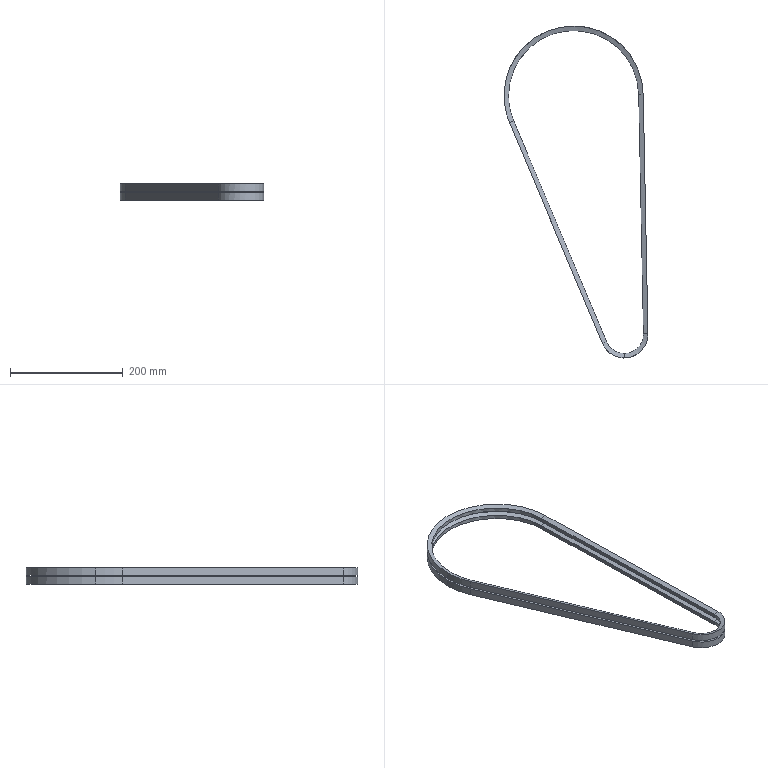Part | SolidWorks | 2 solids | 40 faces | box 255.391 x 589.134 x 28.445 mm | volume 211928 mm3 | plane 16 | cylinder 12 | cone 12 | commonest cylinder face diameters 231.15 x4 247.025 x4 68.168 x2 84.043 x2